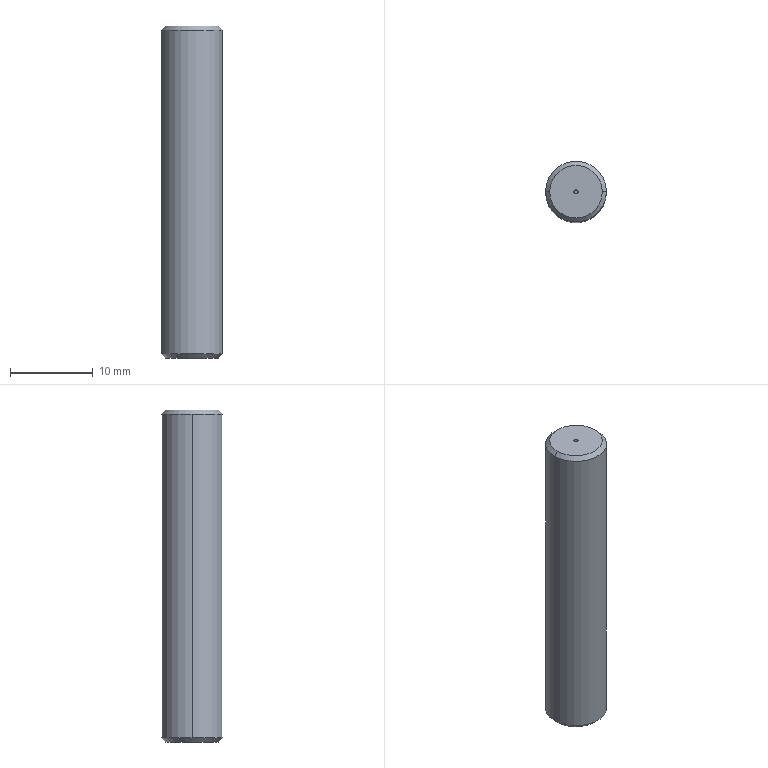Part | SolidWorks | features Chamfer 1, Cut 1, Extrusion 1, MirrorPattern 1 | 1 solid | 14 faces | box 7.349 x 7.349 x 40 mm | volume 1691 mm3 | cone 8 | plane 4 | cylinder 2 | commonest cylinder face diameters 7.349 x2
STEP:
#1=CARTESIAN_POINT('',(-26.868,0.,-19.));
#2=VERTEX_POINT('',#1);
#3=CARTESIAN_POINT('',(-27.263,0.,-19.));
#4=VERTEX_POINT('',#3);
#5=CARTESIAN_POINT('',(-27.066,0.,-19.));
#6=DIRECTION('',(0.,0.,1.));
#7=DIRECTION('',(-1.,0.,0.));
#8=AXIS2_PLACEMENT_3D('',#5,#6,#7);
#9=CIRCLE('',#8,0.1976);
#10=EDGE_CURVE('',#2,#4,#9,.T.);
#11=ORIENTED_EDGE('',*,*,#10,.T.);
#12=CARTESIAN_POINT('',(-27.316,0.,-20.));
#13=VERTEX_POINT('',#12);
#14=CARTESIAN_POINT('',(-27.316,0.,-20.));
#15=DIRECTION('',(-0.05234,0.,-0.9986));
#16=VECTOR('',#15,1000.);
#17=LINE('',#14,#16);
#18=EDGE_CURVE('',#4,#13,#17,.T.);
#19=ORIENTED_EDGE('',*,*,#18,.T.);
#20=CARTESIAN_POINT('',(-26.816,0.,-20.));
#21=VERTEX_POINT('',#20);
#22=CARTESIAN_POINT('',(-27.066,0.,-20.));
#23=DIRECTION('',(0.,0.,1.));
#24=DIRECTION('',(1.,0.,0.));
#25=AXIS2_PLACEMENT_3D('',#22,#23,#24);
#26=CIRCLE('',#25,0.25);
#27=EDGE_CURVE('',#21,#13,#26,.T.);
#28=ORIENTED_EDGE('',*,*,#27,.F.);
#29=CARTESIAN_POINT('',(-26.816,0.,-20.));
#30=DIRECTION('',(0.05234,0.,-0.9986));
#31=VECTOR('',#30,1000.);
#32=LINE('',#29,#31);
#33=EDGE_CURVE('',#2,#21,#32,.T.);
#34=ORIENTED_EDGE('',*,*,#33,.F.);
#35=EDGE_LOOP('',(#11,#19,#28,#34));
#36=FACE_OUTER_BOUND('',#35,.T.);
#37=CARTESIAN_POINT('',(-27.066,0.,-20.));
#38=DIRECTION('',(0.,0.,-1.));
#39=DIRECTION('',(1.,0.,0.));
#40=AXIS2_PLACEMENT_3D('',#37,#38,#39);
#41=CONICAL_SURFACE('',#40,0.25,0.05236);
#42=ADVANCED_FACE('',(#36),#41,.F.);
#43=CARTESIAN_POINT('',(-27.263,0.,19.));
#44=VERTEX_POINT('',#43);
#45=CARTESIAN_POINT('',(-26.868,0.,19.));
#46=VERTEX_POINT('',#45);
#47=CARTESIAN_POINT('',(-27.066,0.,19.));
#48=DIRECTION('',(0.,0.,1.));
#49=DIRECTION('',(1.,0.,0.));
#50=AXIS2_PLACEMENT_3D('',#47,#48,#49);
#51=CIRCLE('',#50,0.1976);
#52=EDGE_CURVE('',#44,#46,#51,.T.);
#53=ORIENTED_EDGE('',*,*,#52,.F.);
#54=CARTESIAN_POINT('',(-27.316,0.,20.));
#55=VERTEX_POINT('',#54);
#56=CARTESIAN_POINT('',(-27.316,0.,20.));
#57=DIRECTION('',(-0.05234,0.,0.9986));
#58=VECTOR('',#57,1000.);
#59=LINE('',#56,#58);
#60=EDGE_CURVE('',#44,#55,#59,.T.);
#61=ORIENTED_EDGE('',*,*,#60,.T.);
#62=CARTESIAN_POINT('',(-26.816,0.,20.));
#63=VERTEX_POINT('',#62);
#64=CARTESIAN_POINT('',(-27.066,0.,20.));
#65=DIRECTION('',(0.,0.,1.));
#66=DIRECTION('',(1.,0.,0.));
#67=AXIS2_PLACEMENT_3D('',#64,#65,#66);
#68=CIRCLE('',#67,0.25);
#69=EDGE_CURVE('',#55,#63,#68,.T.);
#70=ORIENTED_EDGE('',*,*,#69,.T.);
#71=CARTESIAN_POINT('',(-26.816,0.,20.));
#72=DIRECTION('',(0.05234,0.,0.9986));
#73=VECTOR('',#72,1000.);
#74=LINE('',#71,#73);
#75=EDGE_CURVE('',#46,#63,#74,.T.);
#76=ORIENTED_EDGE('',*,*,#75,.F.);
#77=EDGE_LOOP('',(#53,#61,#70,#76));
#78=FACE_OUTER_BOUND('',#77,.T.);
#79=CARTESIAN_POINT('',(-27.066,0.,20.));
#80=DIRECTION('',(0.,0.,1.));
#81=DIRECTION('',(1.,0.,0.));
#82=AXIS2_PLACEMENT_3D('',#79,#80,#81);
#83=CONICAL_SURFACE('',#82,0.25,0.05236);
#84=ADVANCED_FACE('',(#78),#83,.F.);
#85=CARTESIAN_POINT('',(-23.891,0.,20.));
#86=VERTEX_POINT('',#85);
#87=CARTESIAN_POINT('',(-30.24,0.,20.));
#88=VERTEX_POINT('',#87);
#89=CARTESIAN_POINT('',(-27.066,0.,20.));
#90=DIRECTION('',(0.,0.,1.));
#91=DIRECTION('',(1.,0.,0.));
#92=AXIS2_PLACEMENT_3D('',#89,#90,#91);
#93=CIRCLE('',#92,3.175);
#94=EDGE_CURVE('',#86,#88,#93,.T.);
#95=ORIENTED_EDGE('',*,*,#94,.F.);
#96=CARTESIAN_POINT('',(-23.391,0.,19.5));
#97=VERTEX_POINT('',#96);
#98=CARTESIAN_POINT('',(-23.891,0.,20.));
#99=DIRECTION('',(0.7071,0.,-0.7071));
#100=VECTOR('',#99,1000.);
#101=LINE('',#98,#100);
#102=EDGE_CURVE('',#86,#97,#101,.T.);
#103=ORIENTED_EDGE('',*,*,#102,.T.);
#104=CARTESIAN_POINT('',(-30.74,0.,19.5));
#105=VERTEX_POINT('',#104);
#106=CARTESIAN_POINT('',(-27.066,0.,19.5));
#107=DIRECTION('',(0.,0.,-1.));
#108=DIRECTION('',(1.,0.,0.));
#109=AXIS2_PLACEMENT_3D('',#106,#107,#108);
#110=CIRCLE('',#109,3.675);
#111=EDGE_CURVE('',#105,#97,#110,.T.);
#112=ORIENTED_EDGE('',*,*,#111,.F.);
#113=CARTESIAN_POINT('',(-30.24,0.,20.));
#114=DIRECTION('',(-0.7071,0.,-0.7071));
#115=VECTOR('',#114,1000.);
#116=LINE('',#113,#115);
#117=EDGE_CURVE('',#88,#105,#116,.T.);
#118=ORIENTED_EDGE('',*,*,#117,.F.);
#119=EDGE_LOOP('',(#95,#103,#112,#118));
#120=FACE_OUTER_BOUND('',#119,.T.);
#121=CARTESIAN_POINT('',(-27.066,0.,20.));
#122=DIRECTION('',(0.,0.,-1.));
#123=DIRECTION('',(-1.,0.,0.));
#124=AXIS2_PLACEMENT_3D('',#121,#122,#123);
#125=CONICAL_SURFACE('',#124,3.175,0.7854);
#126=ADVANCED_FACE('',(#120),#125,.T.);
#127=CARTESIAN_POINT('',(-30.24,0.,-20.));
#128=VERTEX_POINT('',#127);
#129=CARTESIAN_POINT('',(-23.891,0.,-20.));
#130=VERTEX_POINT('',#129);
#131=CARTESIAN_POINT('',(-27.066,0.,-20.));
#132=DIRECTION('',(0.,0.,-1.));
#133=DIRECTION('',(1.,0.,0.));
#134=AXIS2_PLACEMENT_3D('',#131,#132,#133);
#135=CIRCLE('',#134,3.175);
#136=EDGE_CURVE('',#128,#130,#135,.T.);
#137=ORIENTED_EDGE('',*,*,#136,.F.);
#138=CARTESIAN_POINT('',(-30.74,0.,-19.5));
#139=VERTEX_POINT('',#138);
#140=CARTESIAN_POINT('',(-30.74,0.,-19.5));
#141=DIRECTION('',(-0.7071,0.,0.7071));
#142=VECTOR('',#141,1000.);
#143=LINE('',#140,#142);
#144=EDGE_CURVE('',#128,#139,#143,.T.);
#145=ORIENTED_EDGE('',*,*,#144,.T.);
#146=CARTESIAN_POINT('',(-23.391,0.,-19.5));
#147=VERTEX_POINT('',#146);
#148=CARTESIAN_POINT('',(-27.066,0.,-19.5));
#149=DIRECTION('',(0.,0.,1.));
#150=DIRECTION('',(1.,0.,0.));
#151=AXIS2_PLACEMENT_3D('',#148,#149,#150);
#152=CIRCLE('',#151,3.675);
#153=EDGE_CURVE('',#147,#139,#152,.T.);
#154=ORIENTED_EDGE('',*,*,#153,.F.);
#155=CARTESIAN_POINT('',(-23.391,0.,-19.5));
#156=DIRECTION('',(0.7071,0.,0.7071));
#157=VECTOR('',#156,1000.);
#158=LINE('',#155,#157);
#159=EDGE_CURVE('',#130,#147,#158,.T.);
#160=ORIENTED_EDGE('',*,*,#159,.F.);
#161=EDGE_LOOP('',(#137,#145,#154,#160));
#162=FACE_OUTER_BOUND('',#161,.T.);
#163=CARTESIAN_POINT('',(-27.066,0.,-19.5));
#164=DIRECTION('',(0.,0.,1.));
#165=DIRECTION('',(1.,0.,0.));
#166=AXIS2_PLACEMENT_3D('',#163,#164,#165);
#167=CONICAL_SURFACE('',#166,3.675,0.7854);
#168=ADVANCED_FACE('',(#162),#167,.T.);
#169=ORIENTED_EDGE('',*,*,#111,.T.);
#170=CARTESIAN_POINT('',(-23.391,0.,20.));
#171=DIRECTION('',(0.,0.,-1.));
#172=VECTOR('',#171,1000.);
#173=LINE('',#170,#172);
#174=EDGE_CURVE('',#97,#147,#173,.T.);
#175=ORIENTED_EDGE('',*,*,#174,.T.);
#176=ORIENTED_EDGE('',*,*,#153,.T.);
#177=CARTESIAN_POINT('',(-30.74,0.,20.));
#178=DIRECTION('',(0.,0.,-1.));
#179=VECTOR('',#178,1000.);
#180=LINE('',#177,#179);
#181=EDGE_CURVE('',#105,#139,#180,.T.);
#182=ORIENTED_EDGE('',*,*,#181,.F.);
#183=EDGE_LOOP('',(#169,#175,#176,#182));
#184=FACE_OUTER_BOUND('',#183,.T.);
#185=CARTESIAN_POINT('',(-27.066,0.,20.));
#186=DIRECTION('',(0.,0.,-1.));
#187=DIRECTION('',(-1.,0.,0.));
#188=AXIS2_PLACEMENT_3D('',#185,#186,#187);
#189=CYLINDRICAL_SURFACE('',#188,3.675);
#190=ADVANCED_FACE('',(#184),#189,.T.);
#191=ORIENTED_EDGE('',*,*,#174,.F.);
#192=CARTESIAN_POINT('',(-27.066,0.,19.5));
#193=DIRECTION('',(0.,0.,-1.));
#194=DIRECTION('',(1.,0.,0.));
#195=AXIS2_PLACEMENT_3D('',#192,#193,#194);
#196=CIRCLE('',#195,3.675);
#197=EDGE_CURVE('',#97,#105,#196,.T.);
#198=ORIENTED_EDGE('',*,*,#197,.T.);
#199=ORIENTED_EDGE('',*,*,#181,.T.);
#200=CARTESIAN_POINT('',(-27.066,0.,-19.5));
#201=DIRECTION('',(0.,0.,1.));
#202=DIRECTION('',(1.,0.,0.));
#203=AXIS2_PLACEMENT_3D('',#200,#201,#202);
#204=CIRCLE('',#203,3.675);
#205=EDGE_CURVE('',#139,#147,#204,.T.);
#206=ORIENTED_EDGE('',*,*,#205,.T.);
#207=EDGE_LOOP('',(#191,#198,#199,#206));
#208=FACE_OUTER_BOUND('',#207,.T.);
#209=CARTESIAN_POINT('',(-27.066,0.,20.));
#210=DIRECTION('',(0.,0.,-1.));
#211=DIRECTION('',(-1.,0.,0.));
#212=AXIS2_PLACEMENT_3D('',#209,#210,#211);
#213=CYLINDRICAL_SURFACE('',#212,3.675);
#214=ADVANCED_FACE('',(#208),#213,.T.);
#215=CARTESIAN_POINT('',(-27.066,0.,20.));
#216=DIRECTION('',(0.,0.,1.));
#217=DIRECTION('',(1.,0.,0.));
#218=AXIS2_PLACEMENT_3D('',#215,#216,#217);
#219=CIRCLE('',#218,0.25);
#220=EDGE_CURVE('',#63,#55,#219,.T.);
#221=ORIENTED_EDGE('',*,*,#220,.F.);
#222=ORIENTED_EDGE('',*,*,#69,.F.);
#223=EDGE_LOOP('',(#221,#222));
#224=FACE_BOUND('',#223,.T.);
#225=CARTESIAN_POINT('',(-27.066,0.,20.));
#226=DIRECTION('',(0.,0.,1.));
#227=DIRECTION('',(1.,0.,0.));
#228=AXIS2_PLACEMENT_3D('',#225,#226,#227);
#229=CIRCLE('',#228,3.175);
#230=EDGE_CURVE('',#88,#86,#229,.T.);
#231=ORIENTED_EDGE('',*,*,#230,.T.);
#232=ORIENTED_EDGE('',*,*,#94,.T.);
#233=EDGE_LOOP('',(#231,#232));
#234=FACE_OUTER_BOUND('',#233,.T.);
#235=CARTESIAN_POINT('',(-27.066,0.,20.));
#236=DIRECTION('',(0.,0.,1.));
#237=DIRECTION('',(1.,0.,0.));
#238=AXIS2_PLACEMENT_3D('',#235,#236,#237);
#239=PLANE('',#238);
#240=ADVANCED_FACE('',(#224,#234),#239,.T.);
#241=ORIENTED_EDGE('',*,*,#27,.T.);
#242=CARTESIAN_POINT('',(-27.066,0.,-20.));
#243=DIRECTION('',(0.,0.,1.));
#244=DIRECTION('',(1.,0.,0.));
#245=AXIS2_PLACEMENT_3D('',#242,#243,#244);
#246=CIRCLE('',#245,0.25);
#247=EDGE_CURVE('',#13,#21,#246,.T.);
#248=ORIENTED_EDGE('',*,*,#247,.T.);
#249=EDGE_LOOP('',(#241,#248));
#250=FACE_BOUND('',#249,.T.);
#251=CARTESIAN_POINT('',(-27.066,0.,-20.));
#252=DIRECTION('',(0.,0.,-1.));
#253=DIRECTION('',(1.,0.,0.));
#254=AXIS2_PLACEMENT_3D('',#251,#252,#253);
#255=CIRCLE('',#254,3.175);
#256=EDGE_CURVE('',#130,#128,#255,.T.);
#257=ORIENTED_EDGE('',*,*,#256,.T.);
#258=ORIENTED_EDGE('',*,*,#136,.T.);
#259=EDGE_LOOP('',(#257,#258));
#260=FACE_OUTER_BOUND('',#259,.T.);
#261=CARTESIAN_POINT('',(-27.066,0.,-20.));
#262=DIRECTION('',(0.,0.,1.));
#263=DIRECTION('',(1.,0.,0.));
#264=AXIS2_PLACEMENT_3D('',#261,#262,#263);
#265=PLANE('',#264);
#266=ADVANCED_FACE('',(#250,#260),#265,.F.);
#267=ORIENTED_EDGE('',*,*,#144,.F.);
#268=ORIENTED_EDGE('',*,*,#256,.F.);
#269=ORIENTED_EDGE('',*,*,#159,.T.);
#270=ORIENTED_EDGE('',*,*,#205,.F.);
#271=EDGE_LOOP('',(#267,#268,#269,#270));
#272=FACE_OUTER_BOUND('',#271,.T.);
#273=CARTESIAN_POINT('',(-27.066,0.,-19.5));
#274=DIRECTION('',(0.,0.,1.));
#275=DIRECTION('',(1.,0.,0.));
#276=AXIS2_PLACEMENT_3D('',#273,#274,#275);
#277=CONICAL_SURFACE('',#276,3.675,0.7854);
#278=ADVANCED_FACE('',(#272),#277,.T.);
#279=ORIENTED_EDGE('',*,*,#102,.F.);
#280=ORIENTED_EDGE('',*,*,#230,.F.);
#281=ORIENTED_EDGE('',*,*,#117,.T.);
#282=ORIENTED_EDGE('',*,*,#197,.F.);
#283=EDGE_LOOP('',(#279,#280,#281,#282));
#284=FACE_OUTER_BOUND('',#283,.T.);
#285=CARTESIAN_POINT('',(-27.066,0.,20.));
#286=DIRECTION('',(0.,0.,-1.));
#287=DIRECTION('',(-1.,0.,0.));
#288=AXIS2_PLACEMENT_3D('',#285,#286,#287);
#289=CONICAL_SURFACE('',#288,3.175,0.7854);
#290=ADVANCED_FACE('',(#284),#289,.T.);
#291=ORIENTED_EDGE('',*,*,#60,.F.);
#292=CARTESIAN_POINT('',(-27.066,0.,19.));
#293=DIRECTION('',(0.,0.,1.));
#294=DIRECTION('',(1.,0.,0.));
#295=AXIS2_PLACEMENT_3D('',#292,#293,#294);
#296=CIRCLE('',#295,0.1976);
#297=EDGE_CURVE('',#46,#44,#296,.T.);
#298=ORIENTED_EDGE('',*,*,#297,.F.);
#299=ORIENTED_EDGE('',*,*,#75,.T.);
#300=ORIENTED_EDGE('',*,*,#220,.T.);
#301=EDGE_LOOP('',(#291,#298,#299,#300));
#302=FACE_OUTER_BOUND('',#301,.T.);
#303=CARTESIAN_POINT('',(-27.066,0.,20.));
#304=DIRECTION('',(0.,0.,1.));
#305=DIRECTION('',(1.,0.,0.));
#306=AXIS2_PLACEMENT_3D('',#303,#304,#305);
#307=CONICAL_SURFACE('',#306,0.25,0.05236);
#308=ADVANCED_FACE('',(#302),#307,.F.);
#309=ORIENTED_EDGE('',*,*,#297,.T.);
#310=ORIENTED_EDGE('',*,*,#52,.T.);
#311=EDGE_LOOP('',(#309,#310));
#312=FACE_OUTER_BOUND('',#311,.T.);
#313=CARTESIAN_POINT('',(-27.066,0.,19.));
#314=DIRECTION('',(0.,0.,1.));
#315=DIRECTION('',(1.,0.,0.));
#316=AXIS2_PLACEMENT_3D('',#313,#314,#315);
#317=PLANE('',#316);
#318=ADVANCED_FACE('',(#312),#317,.T.);
#319=ORIENTED_EDGE('',*,*,#18,.F.);
#320=CARTESIAN_POINT('',(-27.066,0.,-19.));
#321=DIRECTION('',(0.,0.,1.));
#322=DIRECTION('',(-1.,0.,0.));
#323=AXIS2_PLACEMENT_3D('',#320,#321,#322);
#324=CIRCLE('',#323,0.1976);
#325=EDGE_CURVE('',#4,#2,#324,.T.);
#326=ORIENTED_EDGE('',*,*,#325,.T.);
#327=ORIENTED_EDGE('',*,*,#33,.T.);
#328=ORIENTED_EDGE('',*,*,#247,.F.);
#329=EDGE_LOOP('',(#319,#326,#327,#328));
#330=FACE_OUTER_BOUND('',#329,.T.);
#331=CARTESIAN_POINT('',(-27.066,0.,-20.));
#332=DIRECTION('',(0.,0.,-1.));
#333=DIRECTION('',(1.,0.,0.));
#334=AXIS2_PLACEMENT_3D('',#331,#332,#333);
#335=CONICAL_SURFACE('',#334,0.25,0.05236);
#336=ADVANCED_FACE('',(#330),#335,.F.);
#337=ORIENTED_EDGE('',*,*,#10,.F.);
#338=ORIENTED_EDGE('',*,*,#325,.F.);
#339=EDGE_LOOP('',(#337,#338));
#340=FACE_OUTER_BOUND('',#339,.T.);
#341=CARTESIAN_POINT('',(-27.066,0.,-19.));
#342=DIRECTION('',(0.,0.,-1.));
#343=DIRECTION('',(1.,0.,0.));
#344=AXIS2_PLACEMENT_3D('',#341,#342,#343);
#345=PLANE('',#344);
#346=ADVANCED_FACE('',(#340),#345,.T.);
#347=CLOSED_SHELL('',(#42,#84,#126,#168,#190,#214,#240,#266,#278,#290,#308,#318,#336,#346));
#348=MANIFOLD_SOLID_BREP('',#347);
#349=CARTESIAN_POINT('',(0.,0.,0.));
#350=DIRECTION('',(0.,0.,1.));
#351=DIRECTION('',(1.,0.,0.));
#352=AXIS2_PLACEMENT_3D('',#349,#350,#351);
#353=(LENGTH_UNIT()NAMED_UNIT(*)SI_UNIT(.MILLI.,.METRE.));
#354=UNCERTAINTY_MEASURE_WITH_UNIT(LENGTH_MEASURE(0.00001),#353,'','');
#355=(NAMED_UNIT(*)PLANE_ANGLE_UNIT()SI_UNIT($,.RADIAN.));
#356=(NAMED_UNIT(*)SI_UNIT($,.STERADIAN.)SOLID_ANGLE_UNIT());
#357=(GEOMETRIC_REPRESENTATION_CONTEXT(3)GLOBAL_UNCERTAINTY_ASSIGNED_CONTEXT((#354))GLOBAL_UNIT_ASSIGNED_CONTEXT((#353,#355,#356))REPRESENTATION_CONTEXT('',''));
#358=ADVANCED_BREP_SHAPE_REPRESENTATION('',(#348,#352),#357);